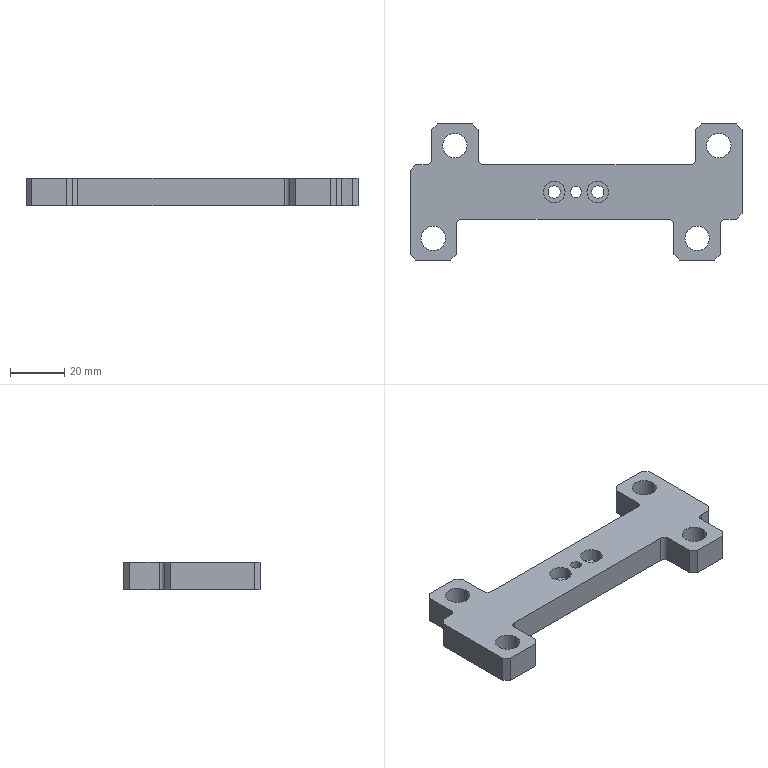Part | STEP file | 08-12 suction plate | 1 solid | 54 faces | box 122 x 50 x 10 mm | volume 31147 mm3 | plane 30 | cylinder 24 | commonest cylinder face diameters 4 x8 9 x8 4.5 x4 8 x4